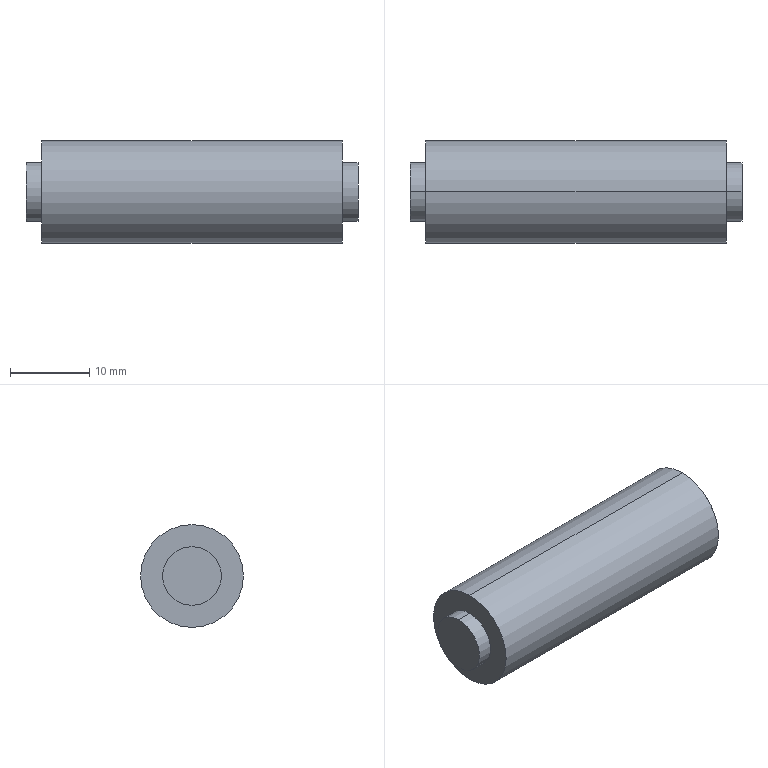Part | SolidWorks | features RefAxis 6, 3DProfileFeature 2, Revolution 1 | 1 solid | 10 faces | box 42 x 13 x 13 mm | volume 5217 mm3 | cylinder 6 | plane 4 | commonest cylinder face diameters 7.429 x4 13 x2
STEP:
#1=CARTESIAN_POINT('',(21.,0.,3.714));
#2=VERTEX_POINT('',#1);
#3=CARTESIAN_POINT('',(21.,0.,-3.714));
#4=VERTEX_POINT('',#3);
#5=CARTESIAN_POINT('',(21.,0.,0.));
#6=DIRECTION('',(-1.,0.,0.));
#7=DIRECTION('',(0.,0.,1.));
#8=AXIS2_PLACEMENT_3D('',#5,#6,#7);
#9=CIRCLE('',#8,3.714);
#10=EDGE_CURVE('',#2,#4,#9,.T.);
#11=ORIENTED_EDGE('',*,*,#10,.T.);
#12=CARTESIAN_POINT('',(19.,0.,-3.714));
#13=VERTEX_POINT('',#12);
#14=CARTESIAN_POINT('',(21.,0.,-3.714));
#15=DIRECTION('',(-1.,0.,0.));
#16=VECTOR('',#15,1000.);
#17=LINE('',#14,#16);
#18=EDGE_CURVE('',#4,#13,#17,.T.);
#19=ORIENTED_EDGE('',*,*,#18,.T.);
#20=CARTESIAN_POINT('',(19.,0.,3.714));
#21=VERTEX_POINT('',#20);
#22=CARTESIAN_POINT('',(19.,0.,0.));
#23=DIRECTION('',(-1.,0.,0.));
#24=DIRECTION('',(0.,0.,1.));
#25=AXIS2_PLACEMENT_3D('',#22,#23,#24);
#26=CIRCLE('',#25,3.714);
#27=EDGE_CURVE('',#21,#13,#26,.T.);
#28=ORIENTED_EDGE('',*,*,#27,.F.);
#29=CARTESIAN_POINT('',(21.,0.,3.714));
#30=DIRECTION('',(-1.,0.,0.));
#31=VECTOR('',#30,1000.);
#32=LINE('',#29,#31);
#33=EDGE_CURVE('',#2,#21,#32,.T.);
#34=ORIENTED_EDGE('',*,*,#33,.F.);
#35=EDGE_LOOP('',(#11,#19,#28,#34));
#36=FACE_OUTER_BOUND('',#35,.T.);
#37=CARTESIAN_POINT('',(21.,0.,0.));
#38=DIRECTION('',(-1.,0.,0.));
#39=DIRECTION('',(0.,0.,1.));
#40=AXIS2_PLACEMENT_3D('',#37,#38,#39);
#41=CYLINDRICAL_SURFACE('',#40,3.714);
#42=ADVANCED_FACE('',(#36),#41,.T.);
#43=CARTESIAN_POINT('',(19.,0.,6.5));
#44=VERTEX_POINT('',#43);
#45=CARTESIAN_POINT('',(19.,0.,-6.5));
#46=VERTEX_POINT('',#45);
#47=CARTESIAN_POINT('',(19.,0.,0.));
#48=DIRECTION('',(-1.,0.,0.));
#49=DIRECTION('',(0.,0.,1.));
#50=AXIS2_PLACEMENT_3D('',#47,#48,#49);
#51=CIRCLE('',#50,6.5);
#52=EDGE_CURVE('',#44,#46,#51,.T.);
#53=ORIENTED_EDGE('',*,*,#52,.T.);
#54=CARTESIAN_POINT('',(-19.,0.,-6.5));
#55=VERTEX_POINT('',#54);
#56=CARTESIAN_POINT('',(21.,0.,-6.5));
#57=DIRECTION('',(-1.,0.,0.));
#58=VECTOR('',#57,1000.);
#59=LINE('',#56,#58);
#60=EDGE_CURVE('',#46,#55,#59,.T.);
#61=ORIENTED_EDGE('',*,*,#60,.T.);
#62=CARTESIAN_POINT('',(-19.,0.,6.5));
#63=VERTEX_POINT('',#62);
#64=CARTESIAN_POINT('',(-19.,0.,0.));
#65=DIRECTION('',(-1.,0.,0.));
#66=DIRECTION('',(0.,0.,1.));
#67=AXIS2_PLACEMENT_3D('',#64,#65,#66);
#68=CIRCLE('',#67,6.5);
#69=EDGE_CURVE('',#63,#55,#68,.T.);
#70=ORIENTED_EDGE('',*,*,#69,.F.);
#71=CARTESIAN_POINT('',(21.,0.,6.5));
#72=DIRECTION('',(-1.,0.,0.));
#73=VECTOR('',#72,1000.);
#74=LINE('',#71,#73);
#75=EDGE_CURVE('',#44,#63,#74,.T.);
#76=ORIENTED_EDGE('',*,*,#75,.F.);
#77=EDGE_LOOP('',(#53,#61,#70,#76));
#78=FACE_OUTER_BOUND('',#77,.T.);
#79=CARTESIAN_POINT('',(21.,0.,0.));
#80=DIRECTION('',(-1.,0.,0.));
#81=DIRECTION('',(0.,0.,1.));
#82=AXIS2_PLACEMENT_3D('',#79,#80,#81);
#83=CYLINDRICAL_SURFACE('',#82,6.5);
#84=ADVANCED_FACE('',(#78),#83,.T.);
#85=CARTESIAN_POINT('',(-19.,0.,3.714));
#86=VERTEX_POINT('',#85);
#87=CARTESIAN_POINT('',(-19.,0.,-3.714));
#88=VERTEX_POINT('',#87);
#89=CARTESIAN_POINT('',(-19.,0.,0.));
#90=DIRECTION('',(-1.,0.,0.));
#91=DIRECTION('',(0.,0.,1.));
#92=AXIS2_PLACEMENT_3D('',#89,#90,#91);
#93=CIRCLE('',#92,3.714);
#94=EDGE_CURVE('',#86,#88,#93,.T.);
#95=ORIENTED_EDGE('',*,*,#94,.T.);
#96=CARTESIAN_POINT('',(-21.,0.,-3.714));
#97=VERTEX_POINT('',#96);
#98=CARTESIAN_POINT('',(21.,0.,-3.714));
#99=DIRECTION('',(-1.,0.,0.));
#100=VECTOR('',#99,1000.);
#101=LINE('',#98,#100);
#102=EDGE_CURVE('',#88,#97,#101,.T.);
#103=ORIENTED_EDGE('',*,*,#102,.T.);
#104=CARTESIAN_POINT('',(-21.,0.,3.714));
#105=VERTEX_POINT('',#104);
#106=CARTESIAN_POINT('',(-21.,0.,0.));
#107=DIRECTION('',(-1.,0.,0.));
#108=DIRECTION('',(0.,0.,1.));
#109=AXIS2_PLACEMENT_3D('',#106,#107,#108);
#110=CIRCLE('',#109,3.714);
#111=EDGE_CURVE('',#105,#97,#110,.T.);
#112=ORIENTED_EDGE('',*,*,#111,.F.);
#113=CARTESIAN_POINT('',(21.,0.,3.714));
#114=DIRECTION('',(-1.,0.,0.));
#115=VECTOR('',#114,1000.);
#116=LINE('',#113,#115);
#117=EDGE_CURVE('',#86,#105,#116,.T.);
#118=ORIENTED_EDGE('',*,*,#117,.F.);
#119=EDGE_LOOP('',(#95,#103,#112,#118));
#120=FACE_OUTER_BOUND('',#119,.T.);
#121=CARTESIAN_POINT('',(21.,0.,0.));
#122=DIRECTION('',(-1.,0.,0.));
#123=DIRECTION('',(0.,0.,1.));
#124=AXIS2_PLACEMENT_3D('',#121,#122,#123);
#125=CYLINDRICAL_SURFACE('',#124,3.714);
#126=ADVANCED_FACE('',(#120),#125,.T.);
#127=ORIENTED_EDGE('',*,*,#111,.T.);
#128=CARTESIAN_POINT('',(-21.,0.,0.));
#129=DIRECTION('',(-1.,0.,0.));
#130=DIRECTION('',(0.,0.,1.));
#131=AXIS2_PLACEMENT_3D('',#128,#129,#130);
#132=CIRCLE('',#131,3.714);
#133=EDGE_CURVE('',#97,#105,#132,.T.);
#134=ORIENTED_EDGE('',*,*,#133,.T.);
#135=EDGE_LOOP('',(#127,#134));
#136=FACE_OUTER_BOUND('',#135,.T.);
#137=CARTESIAN_POINT('',(-21.,0.,0.));
#138=DIRECTION('',(1.,0.,0.));
#139=DIRECTION('',(0.,0.,-1.));
#140=AXIS2_PLACEMENT_3D('',#137,#138,#139);
#141=PLANE('',#140);
#142=ADVANCED_FACE('',(#136),#141,.F.);
#143=ORIENTED_EDGE('',*,*,#102,.F.);
#144=CARTESIAN_POINT('',(-19.,0.,0.));
#145=DIRECTION('',(-1.,0.,0.));
#146=DIRECTION('',(0.,0.,1.));
#147=AXIS2_PLACEMENT_3D('',#144,#145,#146);
#148=CIRCLE('',#147,3.714);
#149=EDGE_CURVE('',#88,#86,#148,.T.);
#150=ORIENTED_EDGE('',*,*,#149,.T.);
#151=ORIENTED_EDGE('',*,*,#117,.T.);
#152=ORIENTED_EDGE('',*,*,#133,.F.);
#153=EDGE_LOOP('',(#143,#150,#151,#152));
#154=FACE_OUTER_BOUND('',#153,.T.);
#155=CARTESIAN_POINT('',(21.,0.,0.));
#156=DIRECTION('',(-1.,0.,0.));
#157=DIRECTION('',(0.,0.,1.));
#158=AXIS2_PLACEMENT_3D('',#155,#156,#157);
#159=CYLINDRICAL_SURFACE('',#158,3.714);
#160=ADVANCED_FACE('',(#154),#159,.T.);
#161=ORIENTED_EDGE('',*,*,#94,.F.);
#162=ORIENTED_EDGE('',*,*,#149,.F.);
#163=EDGE_LOOP('',(#161,#162));
#164=FACE_BOUND('',#163,.T.);
#165=ORIENTED_EDGE('',*,*,#69,.T.);
#166=CARTESIAN_POINT('',(-19.,0.,0.));
#167=DIRECTION('',(-1.,0.,0.));
#168=DIRECTION('',(0.,0.,1.));
#169=AXIS2_PLACEMENT_3D('',#166,#167,#168);
#170=CIRCLE('',#169,6.5);
#171=EDGE_CURVE('',#55,#63,#170,.T.);
#172=ORIENTED_EDGE('',*,*,#171,.T.);
#173=EDGE_LOOP('',(#165,#172));
#174=FACE_OUTER_BOUND('',#173,.T.);
#175=CARTESIAN_POINT('',(-19.,3.714,0.));
#176=DIRECTION('',(1.,0.,0.));
#177=DIRECTION('',(0.,0.,-1.));
#178=AXIS2_PLACEMENT_3D('',#175,#176,#177);
#179=PLANE('',#178);
#180=ADVANCED_FACE('',(#164,#174),#179,.F.);
#181=ORIENTED_EDGE('',*,*,#60,.F.);
#182=CARTESIAN_POINT('',(19.,0.,0.));
#183=DIRECTION('',(-1.,0.,0.));
#184=DIRECTION('',(0.,0.,1.));
#185=AXIS2_PLACEMENT_3D('',#182,#183,#184);
#186=CIRCLE('',#185,6.5);
#187=EDGE_CURVE('',#46,#44,#186,.T.);
#188=ORIENTED_EDGE('',*,*,#187,.T.);
#189=ORIENTED_EDGE('',*,*,#75,.T.);
#190=ORIENTED_EDGE('',*,*,#171,.F.);
#191=EDGE_LOOP('',(#181,#188,#189,#190));
#192=FACE_OUTER_BOUND('',#191,.T.);
#193=CARTESIAN_POINT('',(21.,0.,0.));
#194=DIRECTION('',(-1.,0.,0.));
#195=DIRECTION('',(0.,0.,1.));
#196=AXIS2_PLACEMENT_3D('',#193,#194,#195);
#197=CYLINDRICAL_SURFACE('',#196,6.5);
#198=ADVANCED_FACE('',(#192),#197,.T.);
#199=ORIENTED_EDGE('',*,*,#52,.F.);
#200=ORIENTED_EDGE('',*,*,#187,.F.);
#201=EDGE_LOOP('',(#199,#200));
#202=FACE_OUTER_BOUND('',#201,.T.);
#203=ORIENTED_EDGE('',*,*,#27,.T.);
#204=CARTESIAN_POINT('',(19.,0.,0.));
#205=DIRECTION('',(-1.,0.,0.));
#206=DIRECTION('',(0.,0.,1.));
#207=AXIS2_PLACEMENT_3D('',#204,#205,#206);
#208=CIRCLE('',#207,3.714);
#209=EDGE_CURVE('',#13,#21,#208,.T.);
#210=ORIENTED_EDGE('',*,*,#209,.T.);
#211=EDGE_LOOP('',(#203,#210));
#212=FACE_BOUND('',#211,.T.);
#213=CARTESIAN_POINT('',(19.,6.5,0.));
#214=DIRECTION('',(-1.,0.,0.));
#215=DIRECTION('',(0.,0.,1.));
#216=AXIS2_PLACEMENT_3D('',#213,#214,#215);
#217=PLANE('',#216);
#218=ADVANCED_FACE('',(#202,#212),#217,.F.);
#219=ORIENTED_EDGE('',*,*,#18,.F.);
#220=CARTESIAN_POINT('',(21.,0.,0.));
#221=DIRECTION('',(-1.,0.,0.));
#222=DIRECTION('',(0.,0.,1.));
#223=AXIS2_PLACEMENT_3D('',#220,#221,#222);
#224=CIRCLE('',#223,3.714);
#225=EDGE_CURVE('',#4,#2,#224,.T.);
#226=ORIENTED_EDGE('',*,*,#225,.T.);
#227=ORIENTED_EDGE('',*,*,#33,.T.);
#228=ORIENTED_EDGE('',*,*,#209,.F.);
#229=EDGE_LOOP('',(#219,#226,#227,#228));
#230=FACE_OUTER_BOUND('',#229,.T.);
#231=CARTESIAN_POINT('',(21.,0.,0.));
#232=DIRECTION('',(-1.,0.,0.));
#233=DIRECTION('',(0.,0.,1.));
#234=AXIS2_PLACEMENT_3D('',#231,#232,#233);
#235=CYLINDRICAL_SURFACE('',#234,3.714);
#236=ADVANCED_FACE('',(#230),#235,.T.);
#237=ORIENTED_EDGE('',*,*,#10,.F.);
#238=ORIENTED_EDGE('',*,*,#225,.F.);
#239=EDGE_LOOP('',(#237,#238));
#240=FACE_OUTER_BOUND('',#239,.T.);
#241=CARTESIAN_POINT('',(21.,3.714,0.));
#242=DIRECTION('',(-1.,0.,0.));
#243=DIRECTION('',(0.,0.,1.));
#244=AXIS2_PLACEMENT_3D('',#241,#242,#243);
#245=PLANE('',#244);
#246=ADVANCED_FACE('',(#240),#245,.F.);
#247=CLOSED_SHELL('',(#42,#84,#126,#142,#160,#180,#198,#218,#236,#246));
#248=MANIFOLD_SOLID_BREP('',#247);
#249=CARTESIAN_POINT('',(0.,0.,0.));
#250=DIRECTION('',(0.,0.,1.));
#251=DIRECTION('',(1.,0.,0.));
#252=AXIS2_PLACEMENT_3D('',#249,#250,#251);
#253=(LENGTH_UNIT()NAMED_UNIT(*)SI_UNIT(.MILLI.,.METRE.));
#254=UNCERTAINTY_MEASURE_WITH_UNIT(LENGTH_MEASURE(0.00001),#253,'','');
#255=(NAMED_UNIT(*)PLANE_ANGLE_UNIT()SI_UNIT($,.RADIAN.));
#256=(NAMED_UNIT(*)SI_UNIT($,.STERADIAN.)SOLID_ANGLE_UNIT());
#257=(GEOMETRIC_REPRESENTATION_CONTEXT(3)GLOBAL_UNCERTAINTY_ASSIGNED_CONTEXT((#254))GLOBAL_UNIT_ASSIGNED_CONTEXT((#253,#255,#256))REPRESENTATION_CONTEXT('',''));
#258=ADVANCED_BREP_SHAPE_REPRESENTATION('',(#248,#252),#257);